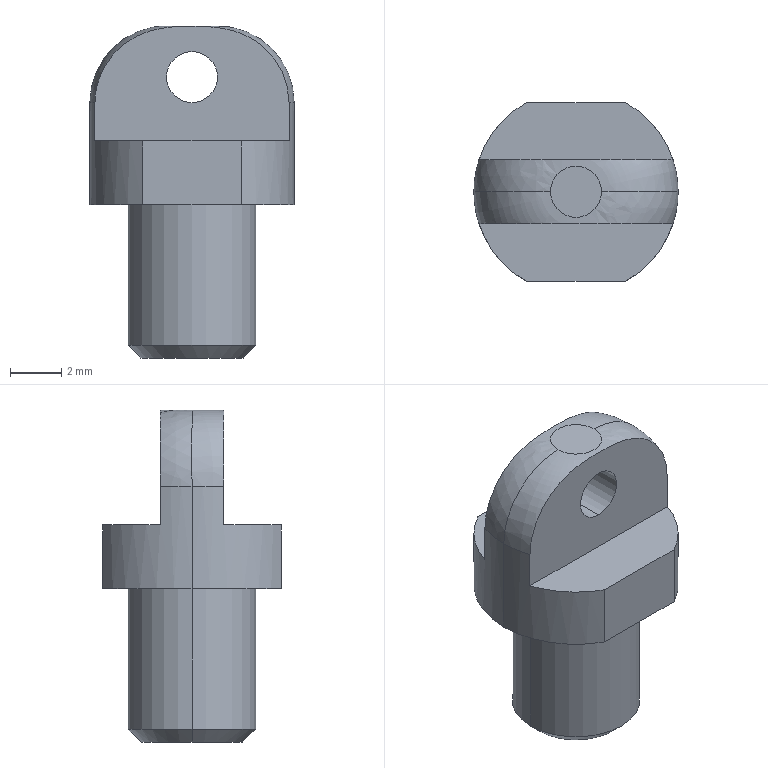Part | STEP file | PN_0039 | 1 solid | 20 faces | box 8 x 7 x 13 mm | volume 305.811 mm3 | plane 9 | cylinder 7 | cone 2 | other 2 | commonest cylinder face diameters 8 x3 2 x2 5 x2